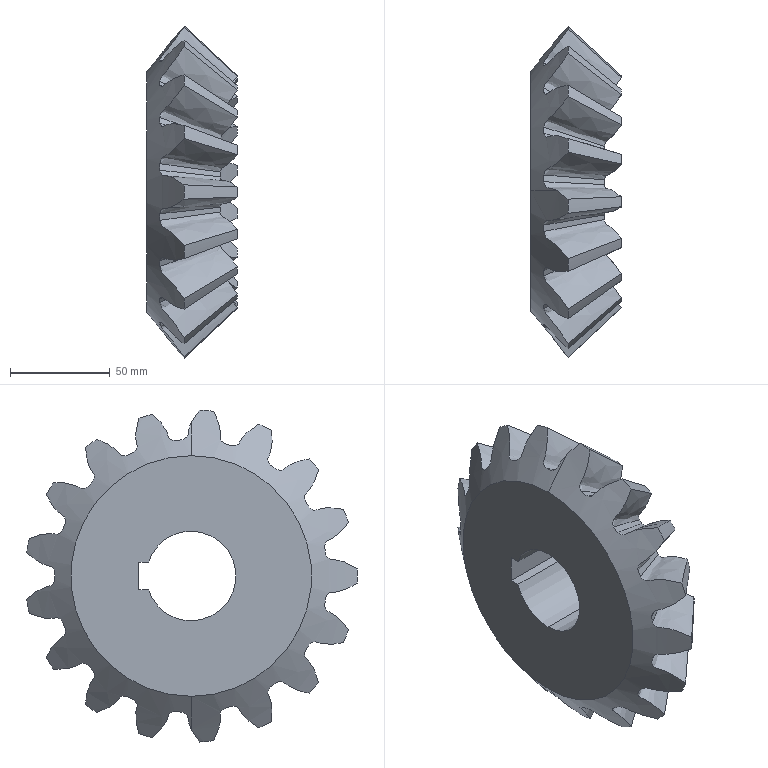Part | SolidWorks | features BlendCut 1, CirPattern 1, ICE 1, RefAxis 1, Revolution 1 | 1 solid | 80 faces | box 45.295 x 166.152 x 166.786 mm | volume 471542 mm3 | spline 51 | cone 21 | plane 5 | cylinder 3 | commonest cylinder face diameters 45 x3